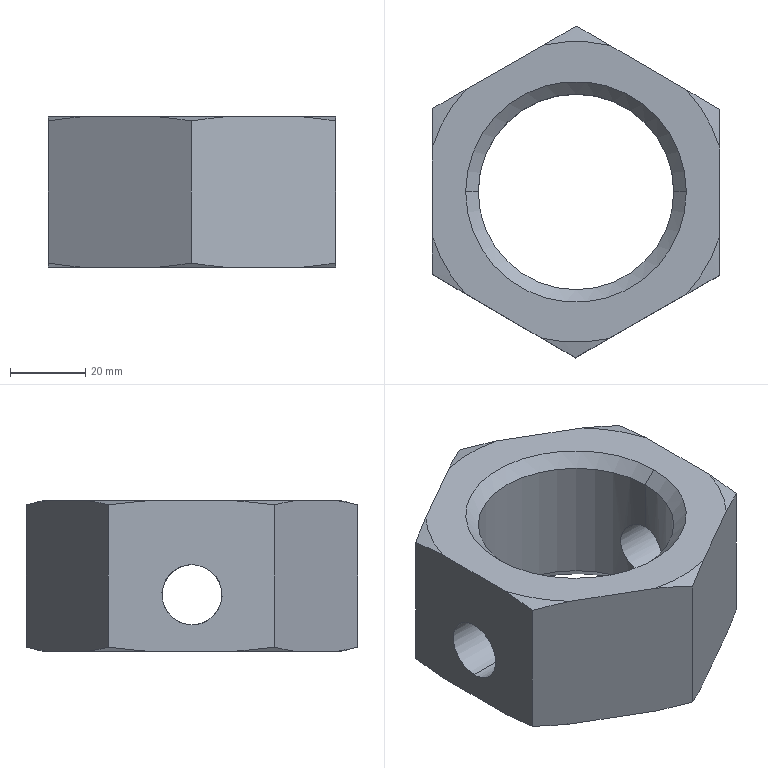Part | NX | features BREP 1 | 1 solid | 30 faces | box 76.6 x 88.249 x 40 mm | volume 110310 mm3 | cone 16 | plane 8 | cylinder 6 | commonest cylinder face diameters 16 x4 52 x2
STEP:
#1=CARTESIAN_POINT('',(-38.214,0.,23.));
#2=VERTEX_POINT('',#1);
#3=CARTESIAN_POINT('',(-38.214,0.,7.));
#4=VERTEX_POINT('',#3);
#5=CARTESIAN_POINT('',(-38.214,0.,23.));
#6=CARTESIAN_POINT('',(-38.277,-16.,23.));
#7=CARTESIAN_POINT('',(-38.277,-16.,7.));
#8=CARTESIAN_POINT('',(-38.214,0.,7.));
#9=(BOUNDED_CURVE()B_SPLINE_CURVE(3,(#5,#6,#7,#8),.UNSPECIFIED.,.F.,.F.)B_SPLINE_CURVE_WITH_KNOTS((4,4),(0.,1.),.PIECEWISE_BEZIER_KNOTS.)CURVE()GEOMETRIC_REPRESENTATION_ITEM()RATIONAL_B_SPLINE_CURVE((1.,0.3333,0.3333,1.))REPRESENTATION_ITEM(''));
#10=EDGE_CURVE('',#2,#4,#9,.T.);
#11=ORIENTED_EDGE('',*,*,#10,.F.);
#12=CARTESIAN_POINT('',(-26.,0.,23.));
#13=VERTEX_POINT('',#12);
#14=CARTESIAN_POINT('',(-60.,0.,23.));
#15=DIRECTION('',(1.,0.,0.));
#16=VECTOR('',#15,1000.);
#17=LINE('',#14,#16);
#18=EDGE_CURVE('',#13,#2,#17,.F.);
#19=ORIENTED_EDGE('',*,*,#18,.F.);
#20=CARTESIAN_POINT('',(-26.,0.,7.));
#21=VERTEX_POINT('',#20);
#22=CARTESIAN_POINT('',(-26.,0.,23.));
#23=CARTESIAN_POINT('',(-26.,-2.127,23.));
#24=CARTESIAN_POINT('',(-25.385,-6.252,21.264));
#25=CARTESIAN_POINT('',(-24.416,-8.873,15.013));
#26=CARTESIAN_POINT('',(-25.384,-6.255,8.732));
#27=CARTESIAN_POINT('',(-26.,-2.128,7.));
#28=CARTESIAN_POINT('',(-26.,0.,7.));
#29=B_SPLINE_CURVE_WITH_KNOTS('',3,(#22,#23,#24,#25,#26,#27,#28),.UNSPECIFIED.,.F.,.F.,(4,1,1,1,4),(0.,0.006289,0.01258,0.01887,0.02516),.UNSPECIFIED.);
#30=EDGE_CURVE('',#13,#21,#29,.T.);
#31=ORIENTED_EDGE('',*,*,#30,.T.);
#32=CARTESIAN_POINT('',(-60.,0.,7.));
#33=DIRECTION('',(1.,0.,0.));
#34=VECTOR('',#33,1000.);
#35=LINE('',#32,#34);
#36=EDGE_CURVE('',#21,#4,#35,.F.);
#37=ORIENTED_EDGE('',*,*,#36,.T.);
#38=EDGE_LOOP('',(#11,#19,#31,#37));
#39=FACE_BOUND('',#38,.T.);
#40=CARTESIAN_POINT('',(-60.,0.,15.));
#41=DIRECTION('',(1.,0.,0.));
#42=DIRECTION('',(0.,0.,1.));
#43=AXIS2_PLACEMENT_3D('',#40,#41,#42);
#44=CYLINDRICAL_SURFACE('',#43,8.);
#45=ADVANCED_FACE('',(#39),#44,.F.);
#46=CARTESIAN_POINT('',(26.,0.,7.));
#47=VERTEX_POINT('',#46);
#48=CARTESIAN_POINT('',(26.,0.,23.));
#49=VERTEX_POINT('',#48);
#50=CARTESIAN_POINT('',(26.,0.,7.));
#51=CARTESIAN_POINT('',(26.,-2.127,7.));
#52=CARTESIAN_POINT('',(25.385,-6.252,8.736));
#53=CARTESIAN_POINT('',(24.416,-8.873,14.987));
#54=CARTESIAN_POINT('',(25.384,-6.255,21.268));
#55=CARTESIAN_POINT('',(26.,-2.128,23.));
#56=CARTESIAN_POINT('',(26.,0.,23.));
#57=B_SPLINE_CURVE_WITH_KNOTS('',3,(#50,#51,#52,#53,#54,#55,#56),.UNSPECIFIED.,.F.,.F.,(4,1,1,1,4),(0.,0.006289,0.01258,0.01887,0.02516),.UNSPECIFIED.);
#58=EDGE_CURVE('',#47,#49,#57,.T.);
#59=ORIENTED_EDGE('',*,*,#58,.T.);
#60=CARTESIAN_POINT('',(38.214,0.,23.));
#61=VERTEX_POINT('',#60);
#62=CARTESIAN_POINT('',(-60.,0.,23.));
#63=DIRECTION('',(1.,0.,0.));
#64=VECTOR('',#63,1000.);
#65=LINE('',#62,#64);
#66=EDGE_CURVE('',#61,#49,#65,.F.);
#67=ORIENTED_EDGE('',*,*,#66,.F.);
#68=CARTESIAN_POINT('',(38.214,0.,7.));
#69=VERTEX_POINT('',#68);
#70=CARTESIAN_POINT('',(38.214,0.,7.));
#71=CARTESIAN_POINT('',(38.151,-16.,7.));
#72=CARTESIAN_POINT('',(38.151,-16.,23.));
#73=CARTESIAN_POINT('',(38.214,0.,23.));
#74=(BOUNDED_CURVE()B_SPLINE_CURVE(3,(#70,#71,#72,#73),.UNSPECIFIED.,.F.,.F.)B_SPLINE_CURVE_WITH_KNOTS((4,4),(0.,1.),.PIECEWISE_BEZIER_KNOTS.)CURVE()GEOMETRIC_REPRESENTATION_ITEM()RATIONAL_B_SPLINE_CURVE((1.,0.3333,0.3333,1.))REPRESENTATION_ITEM(''));
#75=EDGE_CURVE('',#69,#61,#74,.T.);
#76=ORIENTED_EDGE('',*,*,#75,.F.);
#77=CARTESIAN_POINT('',(-60.,0.,7.));
#78=DIRECTION('',(1.,0.,0.));
#79=VECTOR('',#78,1000.);
#80=LINE('',#77,#79);
#81=EDGE_CURVE('',#69,#47,#80,.F.);
#82=ORIENTED_EDGE('',*,*,#81,.T.);
#83=EDGE_LOOP('',(#59,#67,#76,#82));
#84=FACE_BOUND('',#83,.T.);
#85=CARTESIAN_POINT('',(-60.,0.,15.));
#86=DIRECTION('',(1.,0.,0.));
#87=DIRECTION('',(0.,0.,1.));
#88=AXIS2_PLACEMENT_3D('',#85,#86,#87);
#89=CYLINDRICAL_SURFACE('',#88,8.);
#90=ADVANCED_FACE('',(#84),#89,.F.);
#91=CARTESIAN_POINT('',(-26.,0.,36.662));
#92=VERTEX_POINT('',#91);
#93=CARTESIAN_POINT('',(26.,0.,36.662));
#94=VERTEX_POINT('',#93);
#95=CARTESIAN_POINT('',(0.,0.,36.662));
#96=DIRECTION('',(0.,0.,1.));
#97=DIRECTION('',(-1.,0.,0.));
#98=AXIS2_PLACEMENT_3D('',#95,#96,#97);
#99=CIRCLE('',#98,26.);
#100=EDGE_CURVE('',#92,#94,#99,.T.);
#101=ORIENTED_EDGE('',*,*,#100,.F.);
#102=CARTESIAN_POINT('',(-29.338,0.,40.));
#103=VERTEX_POINT('',#102);
#104=CARTESIAN_POINT('',(-26.,0.,36.662));
#105=DIRECTION('',(-0.7071,0.,0.7071));
#106=VECTOR('',#105,1000.);
#107=LINE('',#104,#106);
#108=EDGE_CURVE('',#92,#103,#107,.T.);
#109=ORIENTED_EDGE('',*,*,#108,.T.);
#110=CARTESIAN_POINT('',(29.338,0.,40.));
#111=VERTEX_POINT('',#110);
#112=CARTESIAN_POINT('',(0.,0.,40.));
#113=DIRECTION('',(0.,0.,-1.));
#114=DIRECTION('',(-1.,0.,0.));
#115=AXIS2_PLACEMENT_3D('',#112,#113,#114);
#116=CIRCLE('',#115,29.338);
#117=EDGE_CURVE('',#111,#103,#116,.T.);
#118=ORIENTED_EDGE('',*,*,#117,.F.);
#119=CARTESIAN_POINT('',(26.,0.,36.662));
#120=DIRECTION('',(0.7071,0.,0.7071));
#121=VECTOR('',#120,1000.);
#122=LINE('',#119,#121);
#123=EDGE_CURVE('',#94,#111,#122,.T.);
#124=ORIENTED_EDGE('',*,*,#123,.F.);
#125=EDGE_LOOP('',(#101,#109,#118,#124));
#126=FACE_BOUND('',#125,.T.);
#127=CARTESIAN_POINT('',(0.,0.,36.662));
#128=DIRECTION('',(0.,0.,1.));
#129=DIRECTION('',(-1.,0.,0.));
#130=AXIS2_PLACEMENT_3D('',#127,#128,#129);
#131=CONICAL_SURFACE('',#130,26.,0.7854);
#132=ADVANCED_FACE('',(#126),#131,.F.);
#133=CARTESIAN_POINT('',(26.,0.,3.338));
#134=VERTEX_POINT('',#133);
#135=CARTESIAN_POINT('',(-26.,0.,3.338));
#136=VERTEX_POINT('',#135);
#137=CARTESIAN_POINT('',(0.,0.,3.338));
#138=DIRECTION('',(0.,0.,-1.));
#139=DIRECTION('',(-1.,0.,0.));
#140=AXIS2_PLACEMENT_3D('',#137,#138,#139);
#141=CIRCLE('',#140,26.);
#142=EDGE_CURVE('',#134,#136,#141,.T.);
#143=ORIENTED_EDGE('',*,*,#142,.F.);
#144=CARTESIAN_POINT('',(29.338,0.,0.));
#145=VERTEX_POINT('',#144);
#146=CARTESIAN_POINT('',(29.338,0.,0.));
#147=DIRECTION('',(0.7071,0.,-0.7071));
#148=VECTOR('',#147,1000.);
#149=LINE('',#146,#148);
#150=EDGE_CURVE('',#145,#134,#149,.F.);
#151=ORIENTED_EDGE('',*,*,#150,.F.);
#152=CARTESIAN_POINT('',(-29.338,0.,0.));
#153=VERTEX_POINT('',#152);
#154=CARTESIAN_POINT('',(0.,0.,0.));
#155=DIRECTION('',(0.,0.,1.));
#156=DIRECTION('',(-1.,0.,0.));
#157=AXIS2_PLACEMENT_3D('',#154,#155,#156);
#158=CIRCLE('',#157,29.338);
#159=EDGE_CURVE('',#153,#145,#158,.T.);
#160=ORIENTED_EDGE('',*,*,#159,.F.);
#161=CARTESIAN_POINT('',(-29.338,0.,0.));
#162=DIRECTION('',(-0.7071,0.,-0.7071));
#163=VECTOR('',#162,1000.);
#164=LINE('',#161,#163);
#165=EDGE_CURVE('',#153,#136,#164,.F.);
#166=ORIENTED_EDGE('',*,*,#165,.T.);
#167=EDGE_LOOP('',(#143,#151,#160,#166));
#168=FACE_BOUND('',#167,.T.);
#169=CARTESIAN_POINT('',(0.,0.,0.));
#170=DIRECTION('',(0.,0.,-1.));
#171=DIRECTION('',(1.,0.,0.));
#172=AXIS2_PLACEMENT_3D('',#169,#170,#171);
#173=CONICAL_SURFACE('',#172,29.338,0.7854);
#174=ADVANCED_FACE('',(#168),#173,.F.);
#175=ORIENTED_EDGE('',*,*,#100,.T.);
#176=CARTESIAN_POINT('',(26.,0.,40.));
#177=DIRECTION('',(0.,0.,-1.));
#178=VECTOR('',#177,1000.);
#179=LINE('',#176,#178);
#180=EDGE_CURVE('',#49,#94,#179,.F.);
#181=ORIENTED_EDGE('',*,*,#180,.F.);
#182=ORIENTED_EDGE('',*,*,#58,.F.);
#183=CARTESIAN_POINT('',(26.,0.,40.));
#184=DIRECTION('',(0.,0.,-1.));
#185=VECTOR('',#184,1000.);
#186=LINE('',#183,#185);
#187=EDGE_CURVE('',#134,#47,#186,.F.);
#188=ORIENTED_EDGE('',*,*,#187,.F.);
#189=ORIENTED_EDGE('',*,*,#142,.T.);
#190=CARTESIAN_POINT('',(-26.,0.,40.));
#191=DIRECTION('',(0.,0.,-1.));
#192=VECTOR('',#191,1000.);
#193=LINE('',#190,#192);
#194=EDGE_CURVE('',#136,#21,#193,.F.);
#195=ORIENTED_EDGE('',*,*,#194,.T.);
#196=ORIENTED_EDGE('',*,*,#30,.F.);
#197=CARTESIAN_POINT('',(-26.,0.,40.));
#198=DIRECTION('',(0.,0.,-1.));
#199=VECTOR('',#198,1000.);
#200=LINE('',#197,#199);
#201=EDGE_CURVE('',#13,#92,#200,.F.);
#202=ORIENTED_EDGE('',*,*,#201,.T.);
#203=EDGE_LOOP('',(#175,#181,#182,#188,#189,#195,#196,#202));
#204=FACE_BOUND('',#203,.T.);
#205=CARTESIAN_POINT('',(0.,0.,40.));
#206=DIRECTION('',(0.,0.,-1.));
#207=DIRECTION('',(1.,0.,0.));
#208=AXIS2_PLACEMENT_3D('',#205,#206,#207);
#209=CYLINDRICAL_SURFACE('',#208,26.);
#210=ADVANCED_FACE('',(#204),#209,.F.);
#211=CARTESIAN_POINT('',(38.3,21.912,38.895));
#212=VERTEX_POINT('',#211);
#213=CARTESIAN_POINT('',(29.451,27.068,40.));
#214=VERTEX_POINT('',#213);
#215=CARTESIAN_POINT('',(38.3,21.912,38.895));
#216=CARTESIAN_POINT('',(35.358,23.626,39.351));
#217=CARTESIAN_POINT('',(32.41,25.344,39.729));
#218=CARTESIAN_POINT('',(29.451,27.068,40.));
#219=B_SPLINE_CURVE_WITH_KNOTS('',3,(#215,#216,#217,#218),.UNSPECIFIED.,.F.,.F.,(4,4),(0.,0.0103),.UNSPECIFIED.);
#220=EDGE_CURVE('',#212,#214,#219,.T.);
#221=ORIENTED_EDGE('',*,*,#220,.F.);
#222=CARTESIAN_POINT('',(38.3,21.912,1.105));
#223=VERTEX_POINT('',#222);
#224=CARTESIAN_POINT('',(38.3,21.912,40.));
#225=DIRECTION('',(0.,0.,-1.));
#226=VECTOR('',#225,1000.);
#227=LINE('',#224,#226);
#228=EDGE_CURVE('',#212,#223,#227,.T.);
#229=ORIENTED_EDGE('',*,*,#228,.T.);
#230=CARTESIAN_POINT('',(29.451,27.068,0.));
#231=VERTEX_POINT('',#230);
#232=CARTESIAN_POINT('',(29.451,27.068,0.));
#233=CARTESIAN_POINT('',(32.41,25.344,0.2712));
#234=CARTESIAN_POINT('',(35.358,23.626,0.6492));
#235=CARTESIAN_POINT('',(38.3,21.912,1.105));
#236=B_SPLINE_CURVE_WITH_KNOTS('',3,(#232,#233,#234,#235),.UNSPECIFIED.,.F.,.F.,(4,4),(0.,0.0103),.UNSPECIFIED.);
#237=EDGE_CURVE('',#231,#223,#236,.T.);
#238=ORIENTED_EDGE('',*,*,#237,.F.);
#239=CARTESIAN_POINT('',(9.023,38.969,0.));
#240=VERTEX_POINT('',#239);
#241=CARTESIAN_POINT('',(38.3,21.912,0.));
#242=DIRECTION('',(-0.8641,0.5034,0.));
#243=VECTOR('',#242,1000.);
#244=LINE('',#241,#243);
#245=EDGE_CURVE('',#231,#240,#244,.T.);
#246=ORIENTED_EDGE('',*,*,#245,.T.);
#247=CARTESIAN_POINT('',(0.1736,44.125,1.105));
#248=VERTEX_POINT('',#247);
#249=CARTESIAN_POINT('',(0.1736,44.125,1.105));
#250=CARTESIAN_POINT('',(3.115,42.411,0.6492));
#251=CARTESIAN_POINT('',(6.064,40.693,0.2712));
#252=CARTESIAN_POINT('',(9.023,38.969,0.));
#253=B_SPLINE_CURVE_WITH_KNOTS('',3,(#249,#250,#251,#252),.UNSPECIFIED.,.F.,.F.,(4,4),(0.,0.0103),.UNSPECIFIED.);
#254=EDGE_CURVE('',#248,#240,#253,.T.);
#255=ORIENTED_EDGE('',*,*,#254,.F.);
#256=CARTESIAN_POINT('',(0.1736,44.125,38.895));
#257=VERTEX_POINT('',#256);
#258=CARTESIAN_POINT('',(0.1736,44.125,40.));
#259=DIRECTION('',(0.,0.,-1.));
#260=VECTOR('',#259,1000.);
#261=LINE('',#258,#260);
#262=EDGE_CURVE('',#257,#248,#261,.T.);
#263=ORIENTED_EDGE('',*,*,#262,.F.);
#264=CARTESIAN_POINT('',(9.023,38.969,40.));
#265=VERTEX_POINT('',#264);
#266=CARTESIAN_POINT('',(9.023,38.969,40.));
#267=CARTESIAN_POINT('',(6.064,40.693,39.729));
#268=CARTESIAN_POINT('',(3.115,42.411,39.351));
#269=CARTESIAN_POINT('',(0.1736,44.125,38.895));
#270=B_SPLINE_CURVE_WITH_KNOTS('',3,(#266,#267,#268,#269),.UNSPECIFIED.,.F.,.F.,(4,4),(0.,0.0103),.UNSPECIFIED.);
#271=EDGE_CURVE('',#265,#257,#270,.T.);
#272=ORIENTED_EDGE('',*,*,#271,.F.);
#273=CARTESIAN_POINT('',(38.3,21.912,40.));
#274=DIRECTION('',(-0.8641,0.5034,0.));
#275=VECTOR('',#274,1000.);
#276=LINE('',#273,#275);
#277=EDGE_CURVE('',#214,#265,#276,.T.);
#278=ORIENTED_EDGE('',*,*,#277,.F.);
#279=EDGE_LOOP('',(#221,#229,#238,#246,#255,#263,#272,#278));
#280=FACE_BOUND('',#279,.T.);
#281=CARTESIAN_POINT('',(38.3,21.912,40.));
#282=DIRECTION('',(-0.5034,-0.8641,0.));
#283=DIRECTION('',(-0.8641,0.5034,0.));
#284=AXIS2_PLACEMENT_3D('',#281,#282,#283);
#285=PLANE('',#284);
#286=ADVANCED_FACE('',(#280),#285,.F.);
#287=CARTESIAN_POINT('',(-8.716,39.039,40.));
#288=VERTEX_POINT('',#287);
#289=CARTESIAN_POINT('',(0.1736,44.125,38.895));
#290=CARTESIAN_POINT('',(-2.781,42.434,39.351));
#291=CARTESIAN_POINT('',(-5.744,40.739,39.729));
#292=CARTESIAN_POINT('',(-8.716,39.039,40.));
#293=B_SPLINE_CURVE_WITH_KNOTS('',3,(#289,#290,#291,#292),.UNSPECIFIED.,.F.,.F.,(4,4),(0.,0.0103),.UNSPECIFIED.);
#294=EDGE_CURVE('',#257,#288,#293,.T.);
#295=ORIENTED_EDGE('',*,*,#294,.F.);
#296=ORIENTED_EDGE('',*,*,#262,.T.);
#297=CARTESIAN_POINT('',(-8.716,39.039,0.));
#298=VERTEX_POINT('',#297);
#299=CARTESIAN_POINT('',(-8.716,39.039,0.));
#300=CARTESIAN_POINT('',(-5.744,40.739,0.2712));
#301=CARTESIAN_POINT('',(-2.781,42.434,0.6492));
#302=CARTESIAN_POINT('',(0.1736,44.125,1.105));
#303=B_SPLINE_CURVE_WITH_KNOTS('',3,(#299,#300,#301,#302),.UNSPECIFIED.,.F.,.F.,(4,4),(0.,0.0103),.UNSPECIFIED.);
#304=EDGE_CURVE('',#298,#248,#303,.T.);
#305=ORIENTED_EDGE('',*,*,#304,.F.);
#306=CARTESIAN_POINT('',(-29.237,27.298,0.));
#307=VERTEX_POINT('',#306);
#308=CARTESIAN_POINT('',(0.1736,44.125,0.));
#309=DIRECTION('',(-0.868,-0.4966,0.));
#310=VECTOR('',#309,1000.);
#311=LINE('',#308,#310);
#312=EDGE_CURVE('',#298,#307,#311,.T.);
#313=ORIENTED_EDGE('',*,*,#312,.T.);
#314=CARTESIAN_POINT('',(-38.126,22.213,1.105));
#315=VERTEX_POINT('',#314);
#316=CARTESIAN_POINT('',(-38.126,22.213,1.105));
#317=CARTESIAN_POINT('',(-35.171,23.903,0.6492));
#318=CARTESIAN_POINT('',(-32.209,25.598,0.2712));
#319=CARTESIAN_POINT('',(-29.237,27.298,0.));
#320=B_SPLINE_CURVE_WITH_KNOTS('',3,(#316,#317,#318,#319),.UNSPECIFIED.,.F.,.F.,(4,4),(0.,0.0103),.UNSPECIFIED.);
#321=EDGE_CURVE('',#315,#307,#320,.T.);
#322=ORIENTED_EDGE('',*,*,#321,.F.);
#323=CARTESIAN_POINT('',(-38.126,22.213,38.895));
#324=VERTEX_POINT('',#323);
#325=CARTESIAN_POINT('',(-38.126,22.213,40.));
#326=DIRECTION('',(0.,0.,-1.));
#327=VECTOR('',#326,1000.);
#328=LINE('',#325,#327);
#329=EDGE_CURVE('',#324,#315,#328,.T.);
#330=ORIENTED_EDGE('',*,*,#329,.F.);
#331=CARTESIAN_POINT('',(-29.237,27.298,40.));
#332=VERTEX_POINT('',#331);
#333=CARTESIAN_POINT('',(-29.237,27.298,40.));
#334=CARTESIAN_POINT('',(-32.209,25.598,39.729));
#335=CARTESIAN_POINT('',(-35.171,23.903,39.351));
#336=CARTESIAN_POINT('',(-38.126,22.213,38.895));
#337=B_SPLINE_CURVE_WITH_KNOTS('',3,(#333,#334,#335,#336),.UNSPECIFIED.,.F.,.F.,(4,4),(0.,0.0103),.UNSPECIFIED.);
#338=EDGE_CURVE('',#332,#324,#337,.T.);
#339=ORIENTED_EDGE('',*,*,#338,.F.);
#340=CARTESIAN_POINT('',(0.1736,44.125,40.));
#341=DIRECTION('',(-0.868,-0.4966,0.));
#342=VECTOR('',#341,1000.);
#343=LINE('',#340,#342);
#344=EDGE_CURVE('',#288,#332,#343,.T.);
#345=ORIENTED_EDGE('',*,*,#344,.F.);
#346=EDGE_LOOP('',(#295,#296,#305,#313,#322,#330,#339,#345));
#347=FACE_BOUND('',#346,.T.);
#348=CARTESIAN_POINT('',(0.1736,44.125,40.));
#349=DIRECTION('',(0.4966,-0.868,0.));
#350=DIRECTION('',(-0.868,-0.4966,0.));
#351=AXIS2_PLACEMENT_3D('',#348,#349,#350);
#352=PLANE('',#351);
#353=ADVANCED_FACE('',(#347),#352,.F.);
#354=CARTESIAN_POINT('',(-38.214,0.,7.));
#355=CARTESIAN_POINT('',(-38.151,16.,7.));
#356=CARTESIAN_POINT('',(-38.151,16.,23.));
#357=CARTESIAN_POINT('',(-38.214,0.,23.));
#358=(BOUNDED_CURVE()B_SPLINE_CURVE(3,(#354,#355,#356,#357),.UNSPECIFIED.,.F.,.F.)B_SPLINE_CURVE_WITH_KNOTS((4,4),(0.,1.),.PIECEWISE_BEZIER_KNOTS.)CURVE()GEOMETRIC_REPRESENTATION_ITEM()RATIONAL_B_SPLINE_CURVE((1.,0.3333,0.3333,1.))REPRESENTATION_ITEM(''));
#359=EDGE_CURVE('',#4,#2,#358,.T.);
#360=ORIENTED_EDGE('',*,*,#359,.T.);
#361=ORIENTED_EDGE('',*,*,#10,.T.);
#362=EDGE_LOOP('',(#360,#361));
#363=FACE_BOUND('',#362,.T.);
#364=CARTESIAN_POINT('',(-38.167,11.971,40.));
#365=VERTEX_POINT('',#364);
#366=CARTESIAN_POINT('',(-38.126,22.213,38.895));
#367=CARTESIAN_POINT('',(-38.14,18.808,39.351));
#368=CARTESIAN_POINT('',(-38.153,15.396,39.729));
#369=CARTESIAN_POINT('',(-38.167,11.971,40.));
#370=B_SPLINE_CURVE_WITH_KNOTS('',3,(#366,#367,#368,#369),.UNSPECIFIED.,.F.,.F.,(4,4),(0.,0.0103),.UNSPECIFIED.);
#371=EDGE_CURVE('',#324,#365,#370,.T.);
#372=ORIENTED_EDGE('',*,*,#371,.F.);
#373=ORIENTED_EDGE('',*,*,#329,.T.);
#374=CARTESIAN_POINT('',(-38.167,11.971,0.));
#375=VERTEX_POINT('',#374);
#376=CARTESIAN_POINT('',(-38.167,11.971,0.));
#377=CARTESIAN_POINT('',(-38.153,15.396,0.2712));
#378=CARTESIAN_POINT('',(-38.14,18.808,0.6492));
#379=CARTESIAN_POINT('',(-38.126,22.213,1.105));
#380=B_SPLINE_CURVE_WITH_KNOTS('',3,(#376,#377,#378,#379),.UNSPECIFIED.,.F.,.F.,(4,4),(0.,0.0103),.UNSPECIFIED.);
#381=EDGE_CURVE('',#375,#315,#380,.T.);
#382=ORIENTED_EDGE('',*,*,#381,.F.);
#383=CARTESIAN_POINT('',(-38.26,-11.671,0.));
#384=VERTEX_POINT('',#383);
#385=CARTESIAN_POINT('',(-38.126,22.213,0.));
#386=DIRECTION('',(-0.003934,-1.,0.));
#387=VECTOR('',#386,1000.);
#388=LINE('',#385,#387);
#389=EDGE_CURVE('',#375,#384,#388,.T.);
#390=ORIENTED_EDGE('',*,*,#389,.T.);
#391=CARTESIAN_POINT('',(-38.3,-21.912,1.105));
#392=VERTEX_POINT('',#391);
#393=CARTESIAN_POINT('',(-38.3,-21.912,1.105));
#394=CARTESIAN_POINT('',(-38.286,-18.508,0.6492));
#395=CARTESIAN_POINT('',(-38.273,-15.095,0.2712));
#396=CARTESIAN_POINT('',(-38.26,-11.671,0.));
#397=B_SPLINE_CURVE_WITH_KNOTS('',3,(#393,#394,#395,#396),.UNSPECIFIED.,.F.,.F.,(4,4),(0.,0.0103),.UNSPECIFIED.);
#398=EDGE_CURVE('',#392,#384,#397,.T.);
#399=ORIENTED_EDGE('',*,*,#398,.F.);
#400=CARTESIAN_POINT('',(-38.3,-21.912,38.895));
#401=VERTEX_POINT('',#400);
#402=CARTESIAN_POINT('',(-38.3,-21.912,40.));
#403=DIRECTION('',(0.,0.,-1.));
#404=VECTOR('',#403,1000.);
#405=LINE('',#402,#404);
#406=EDGE_CURVE('',#401,#392,#405,.T.);
#407=ORIENTED_EDGE('',*,*,#406,.F.);
#408=CARTESIAN_POINT('',(-38.26,-11.671,40.));
#409=VERTEX_POINT('',#408);
#410=CARTESIAN_POINT('',(-38.26,-11.671,40.));
#411=CARTESIAN_POINT('',(-38.273,-15.095,39.729));
#412=CARTESIAN_POINT('',(-38.286,-18.508,39.351));
#413=CARTESIAN_POINT('',(-38.3,-21.912,38.895));
#414=B_SPLINE_CURVE_WITH_KNOTS('',3,(#410,#411,#412,#413),.UNSPECIFIED.,.F.,.F.,(4,4),(0.,0.0103),.UNSPECIFIED.);
#415=EDGE_CURVE('',#409,#401,#414,.T.);
#416=ORIENTED_EDGE('',*,*,#415,.F.);
#417=CARTESIAN_POINT('',(-38.126,22.213,40.));
#418=DIRECTION('',(-0.003934,-1.,0.));
#419=VECTOR('',#418,1000.);
#420=LINE('',#417,#419);
#421=EDGE_CURVE('',#365,#409,#420,.T.);
#422=ORIENTED_EDGE('',*,*,#421,.F.);
#423=EDGE_LOOP('',(#372,#373,#382,#390,#399,#407,#416,#422));
#424=FACE_BOUND('',#423,.T.);
#425=CARTESIAN_POINT('',(-38.126,22.213,40.));
#426=DIRECTION('',(1.,-0.003934,0.));
#427=DIRECTION('',(-0.003934,-1.,0.));
#428=AXIS2_PLACEMENT_3D('',#425,#426,#427);
#429=PLANE('',#428);
#430=ADVANCED_FACE('',(#363,#424),#429,.F.);
#431=CARTESIAN_POINT('',(-29.451,-27.068,40.));
#432=VERTEX_POINT('',#431);
#433=CARTESIAN_POINT('',(-38.3,-21.912,38.895));
#434=CARTESIAN_POINT('',(-35.358,-23.626,39.351));
#435=CARTESIAN_POINT('',(-32.41,-25.344,39.729));
#436=CARTESIAN_POINT('',(-29.451,-27.068,40.));
#437=B_SPLINE_CURVE_WITH_KNOTS('',3,(#433,#434,#435,#436),.UNSPECIFIED.,.F.,.F.,(4,4),(0.,0.0103),.UNSPECIFIED.);
#438=EDGE_CURVE('',#401,#432,#437,.T.);
#439=ORIENTED_EDGE('',*,*,#438,.F.);
#440=ORIENTED_EDGE('',*,*,#406,.T.);
#441=CARTESIAN_POINT('',(-29.451,-27.068,0.));
#442=VERTEX_POINT('',#441);
#443=CARTESIAN_POINT('',(-29.451,-27.068,0.));
#444=CARTESIAN_POINT('',(-32.41,-25.344,0.2712));
#445=CARTESIAN_POINT('',(-35.358,-23.626,0.6492));
#446=CARTESIAN_POINT('',(-38.3,-21.912,1.105));
#447=B_SPLINE_CURVE_WITH_KNOTS('',3,(#443,#444,#445,#446),.UNSPECIFIED.,.F.,.F.,(4,4),(0.,0.0103),.UNSPECIFIED.);
#448=EDGE_CURVE('',#442,#392,#447,.T.);
#449=ORIENTED_EDGE('',*,*,#448,.F.);
#450=CARTESIAN_POINT('',(-9.023,-38.969,0.));
#451=VERTEX_POINT('',#450);
#452=CARTESIAN_POINT('',(-38.3,-21.912,0.));
#453=DIRECTION('',(0.8641,-0.5034,0.));
#454=VECTOR('',#453,1000.);
#455=LINE('',#452,#454);
#456=EDGE_CURVE('',#442,#451,#455,.T.);
#457=ORIENTED_EDGE('',*,*,#456,.T.);
#458=CARTESIAN_POINT('',(-0.1736,-44.125,1.105));
#459=VERTEX_POINT('',#458);
#460=CARTESIAN_POINT('',(-0.1736,-44.125,1.105));
#461=CARTESIAN_POINT('',(-3.115,-42.411,0.6492));
#462=CARTESIAN_POINT('',(-6.064,-40.693,0.2712));
#463=CARTESIAN_POINT('',(-9.023,-38.969,0.));
#464=B_SPLINE_CURVE_WITH_KNOTS('',3,(#460,#461,#462,#463),.UNSPECIFIED.,.F.,.F.,(4,4),(0.,0.0103),.UNSPECIFIED.);
#465=EDGE_CURVE('',#459,#451,#464,.T.);
#466=ORIENTED_EDGE('',*,*,#465,.F.);
#467=CARTESIAN_POINT('',(-0.1736,-44.125,38.895));
#468=VERTEX_POINT('',#467);
#469=CARTESIAN_POINT('',(-0.1736,-44.125,40.));
#470=DIRECTION('',(0.,0.,-1.));
#471=VECTOR('',#470,1000.);
#472=LINE('',#469,#471);
#473=EDGE_CURVE('',#468,#459,#472,.T.);
#474=ORIENTED_EDGE('',*,*,#473,.F.);
#475=CARTESIAN_POINT('',(-9.023,-38.969,40.));
#476=VERTEX_POINT('',#475);
#477=CARTESIAN_POINT('',(-9.023,-38.969,40.));
#478=CARTESIAN_POINT('',(-6.064,-40.693,39.729));
#479=CARTESIAN_POINT('',(-3.115,-42.411,39.351));
#480=CARTESIAN_POINT('',(-0.1736,-44.125,38.895));
#481=B_SPLINE_CURVE_WITH_KNOTS('',3,(#477,#478,#479,#480),.UNSPECIFIED.,.F.,.F.,(4,4),(0.,0.0103),.UNSPECIFIED.);
#482=EDGE_CURVE('',#476,#468,#481,.T.);
#483=ORIENTED_EDGE('',*,*,#482,.F.);
#484=CARTESIAN_POINT('',(-38.3,-21.912,40.));
#485=DIRECTION('',(0.8641,-0.5034,0.));
#486=VECTOR('',#485,1000.);
#487=LINE('',#484,#486);
#488=EDGE_CURVE('',#432,#476,#487,.T.);
#489=ORIENTED_EDGE('',*,*,#488,.F.);
#490=EDGE_LOOP('',(#439,#440,#449,#457,#466,#474,#483,#489));
#491=FACE_BOUND('',#490,.T.);
#492=CARTESIAN_POINT('',(-38.3,-21.912,40.));
#493=DIRECTION('',(0.5034,0.8641,0.));
#494=DIRECTION('',(0.8641,-0.5034,0.));
#495=AXIS2_PLACEMENT_3D('',#492,#493,#494);
#496=PLANE('',#495);
#497=ADVANCED_FACE('',(#491),#496,.F.);
#498=CARTESIAN_POINT('',(8.716,-39.039,40.));
#499=VERTEX_POINT('',#498);
#500=CARTESIAN_POINT('',(-0.1736,-44.125,38.895));
#501=CARTESIAN_POINT('',(2.781,-42.434,39.351));
#502=CARTESIAN_POINT('',(5.744,-40.739,39.729));
#503=CARTESIAN_POINT('',(8.716,-39.039,40.));
#504=B_SPLINE_CURVE_WITH_KNOTS('',3,(#500,#501,#502,#503),.UNSPECIFIED.,.F.,.F.,(4,4),(0.,0.0103),.UNSPECIFIED.);
#505=EDGE_CURVE('',#468,#499,#504,.T.);
#506=ORIENTED_EDGE('',*,*,#505,.F.);
#507=ORIENTED_EDGE('',*,*,#473,.T.);
#508=CARTESIAN_POINT('',(8.716,-39.039,0.));
#509=VERTEX_POINT('',#508);
#510=CARTESIAN_POINT('',(8.716,-39.039,0.));
#511=CARTESIAN_POINT('',(5.744,-40.739,0.2712));
#512=CARTESIAN_POINT('',(2.781,-42.434,0.6492));
#513=CARTESIAN_POINT('',(-0.1736,-44.125,1.105));
#514=B_SPLINE_CURVE_WITH_KNOTS('',3,(#510,#511,#512,#513),.UNSPECIFIED.,.F.,.F.,(4,4),(0.,0.0103),.UNSPECIFIED.);
#515=EDGE_CURVE('',#509,#459,#514,.T.);
#516=ORIENTED_EDGE('',*,*,#515,.F.);
#517=CARTESIAN_POINT('',(29.237,-27.298,0.));
#518=VERTEX_POINT('',#517);
#519=CARTESIAN_POINT('',(-0.1736,-44.125,0.));
#520=DIRECTION('',(0.868,0.4966,0.));
#521=VECTOR('',#520,1000.);
#522=LINE('',#519,#521);
#523=EDGE_CURVE('',#509,#518,#522,.T.);
#524=ORIENTED_EDGE('',*,*,#523,.T.);
#525=CARTESIAN_POINT('',(38.126,-22.213,1.105));
#526=VERTEX_POINT('',#525);
#527=CARTESIAN_POINT('',(38.126,-22.213,1.105));
#528=CARTESIAN_POINT('',(35.171,-23.903,0.6492));
#529=CARTESIAN_POINT('',(32.209,-25.598,0.2712));
#530=CARTESIAN_POINT('',(29.237,-27.298,0.));
#531=B_SPLINE_CURVE_WITH_KNOTS('',3,(#527,#528,#529,#530),.UNSPECIFIED.,.F.,.F.,(4,4),(0.,0.0103),.UNSPECIFIED.);
#532=EDGE_CURVE('',#526,#518,#531,.T.);
#533=ORIENTED_EDGE('',*,*,#532,.F.);
#534=CARTESIAN_POINT('',(38.126,-22.213,38.895));
#535=VERTEX_POINT('',#534);
#536=CARTESIAN_POINT('',(38.126,-22.213,40.));
#537=DIRECTION('',(0.,0.,-1.));
#538=VECTOR('',#537,1000.);
#539=LINE('',#536,#538);
#540=EDGE_CURVE('',#535,#526,#539,.T.);
#541=ORIENTED_EDGE('',*,*,#540,.F.);
#542=CARTESIAN_POINT('',(29.237,-27.298,40.));
#543=VERTEX_POINT('',#542);
#544=CARTESIAN_POINT('',(29.237,-27.298,40.));
#545=CARTESIAN_POINT('',(32.209,-25.598,39.729));
#546=CARTESIAN_POINT('',(35.171,-23.903,39.351));
#547=CARTESIAN_POINT('',(38.126,-22.213,38.895));
#548=B_SPLINE_CURVE_WITH_KNOTS('',3,(#544,#545,#546,#547),.UNSPECIFIED.,.F.,.F.,(4,4),(0.,0.0103),.UNSPECIFIED.);
#549=EDGE_CURVE('',#543,#535,#548,.T.);
#550=ORIENTED_EDGE('',*,*,#549,.F.);
#551=CARTESIAN_POINT('',(-0.1736,-44.125,40.));
#552=DIRECTION('',(0.868,0.4966,0.));
#553=VECTOR('',#552,1000.);
#554=LINE('',#551,#553);
#555=EDGE_CURVE('',#499,#543,#554,.T.);
#556=ORIENTED_EDGE('',*,*,#555,.F.);
#557=EDGE_LOOP('',(#506,#507,#516,#524,#533,#541,#550,#556));
#558=FACE_BOUND('',#557,.T.);
#559=CARTESIAN_POINT('',(-0.1736,-44.125,40.));
#560=DIRECTION('',(-0.4966,0.868,0.));
#561=DIRECTION('',(0.868,0.4966,0.));
#562=AXIS2_PLACEMENT_3D('',#559,#560,#561);
#563=PLANE('',#562);
#564=ADVANCED_FACE('',(#558),#563,.F.);
#565=ORIENTED_EDGE('',*,*,#75,.T.);
#566=CARTESIAN_POINT('',(38.214,0.,23.));
#567=CARTESIAN_POINT('',(38.277,16.,23.));
#568=CARTESIAN_POINT('',(38.277,16.,7.));
#569=CARTESIAN_POINT('',(38.214,0.,7.));
#570=(BOUNDED_CURVE()B_SPLINE_CURVE(3,(#566,#567,#568,#569),.UNSPECIFIED.,.F.,.F.)B_SPLINE_CURVE_WITH_KNOTS((4,4),(0.,1.),.PIECEWISE_BEZIER_KNOTS.)CURVE()GEOMETRIC_REPRESENTATION_ITEM()RATIONAL_B_SPLINE_CURVE((1.,0.3333,0.3333,1.))REPRESENTATION_ITEM(''));
#571=EDGE_CURVE('',#61,#69,#570,.T.);
#572=ORIENTED_EDGE('',*,*,#571,.T.);
#573=EDGE_LOOP('',(#565,#572));
#574=FACE_BOUND('',#573,.T.);
#575=CARTESIAN_POINT('',(38.167,-11.971,40.));
#576=VERTEX_POINT('',#575);
#577=CARTESIAN_POINT('',(38.126,-22.213,38.895));
#578=CARTESIAN_POINT('',(38.14,-18.808,39.351));
#579=CARTESIAN_POINT('',(38.153,-15.396,39.729));
#580=CARTESIAN_POINT('',(38.167,-11.971,40.));
#581=B_SPLINE_CURVE_WITH_KNOTS('',3,(#577,#578,#579,#580),.UNSPECIFIED.,.F.,.F.,(4,4),(0.,0.0103),.UNSPECIFIED.);
#582=EDGE_CURVE('',#535,#576,#581,.T.);
#583=ORIENTED_EDGE('',*,*,#582,.F.);
#584=ORIENTED_EDGE('',*,*,#540,.T.);
#585=CARTESIAN_POINT('',(38.167,-11.971,0.));
#586=VERTEX_POINT('',#585);
#587=CARTESIAN_POINT('',(38.167,-11.971,0.));
#588=CARTESIAN_POINT('',(38.153,-15.396,0.2712));
#589=CARTESIAN_POINT('',(38.14,-18.808,0.6492));
#590=CARTESIAN_POINT('',(38.126,-22.213,1.105));
#591=B_SPLINE_CURVE_WITH_KNOTS('',3,(#587,#588,#589,#590),.UNSPECIFIED.,.F.,.F.,(4,4),(0.,0.0103),.UNSPECIFIED.);
#592=EDGE_CURVE('',#586,#526,#591,.T.);
#593=ORIENTED_EDGE('',*,*,#592,.F.);
#594=CARTESIAN_POINT('',(38.26,11.671,0.));
#595=VERTEX_POINT('',#594);
#596=CARTESIAN_POINT('',(38.126,-22.213,0.));
#597=DIRECTION('',(0.003934,1.,0.));
#598=VECTOR('',#597,1000.);
#599=LINE('',#596,#598);
#600=EDGE_CURVE('',#586,#595,#599,.T.);
#601=ORIENTED_EDGE('',*,*,#600,.T.);
#602=CARTESIAN_POINT('',(38.3,21.912,1.105));
#603=CARTESIAN_POINT('',(38.286,18.508,0.6492));
#604=CARTESIAN_POINT('',(38.273,15.095,0.2712));
#605=CARTESIAN_POINT('',(38.26,11.671,0.));
#606=B_SPLINE_CURVE_WITH_KNOTS('',3,(#602,#603,#604,#605),.UNSPECIFIED.,.F.,.F.,(4,4),(0.,0.0103),.UNSPECIFIED.);
#607=EDGE_CURVE('',#223,#595,#606,.T.);
#608=ORIENTED_EDGE('',*,*,#607,.F.);
#609=ORIENTED_EDGE('',*,*,#228,.F.);
#610=CARTESIAN_POINT('',(38.26,11.671,40.));
#611=VERTEX_POINT('',#610);
#612=CARTESIAN_POINT('',(38.26,11.671,40.));
#613=CARTESIAN_POINT('',(38.273,15.095,39.729));
#614=CARTESIAN_POINT('',(38.286,18.508,39.351));
#615=CARTESIAN_POINT('',(38.3,21.912,38.895));
#616=B_SPLINE_CURVE_WITH_KNOTS('',3,(#612,#613,#614,#615),.UNSPECIFIED.,.F.,.F.,(4,4),(0.,0.0103),.UNSPECIFIED.);
#617=EDGE_CURVE('',#611,#212,#616,.T.);
#618=ORIENTED_EDGE('',*,*,#617,.F.);
#619=CARTESIAN_POINT('',(38.126,-22.213,40.));
#620=DIRECTION('',(0.003934,1.,0.));
#621=VECTOR('',#620,1000.);
#622=LINE('',#619,#621);
#623=EDGE_CURVE('',#576,#611,#622,.T.);
#624=ORIENTED_EDGE('',*,*,#623,.F.);
#625=EDGE_LOOP('',(#583,#584,#593,#601,#608,#609,#618,#624));
#626=FACE_BOUND('',#625,.T.);
#627=CARTESIAN_POINT('',(38.126,-22.213,40.));
#628=DIRECTION('',(-1.,0.003934,0.));
#629=DIRECTION('',(0.003934,1.,0.));
#630=AXIS2_PLACEMENT_3D('',#627,#628,#629);
#631=PLANE('',#630);
#632=ADVANCED_FACE('',(#574,#626),#631,.F.);
#633=ORIENTED_EDGE('',*,*,#117,.T.);
#634=CARTESIAN_POINT('',(0.,0.,40.));
#635=DIRECTION('',(0.,0.,-1.));
#636=DIRECTION('',(-1.,0.,0.));
#637=AXIS2_PLACEMENT_3D('',#634,#635,#636);
#638=CIRCLE('',#637,29.338);
#639=EDGE_CURVE('',#103,#111,#638,.T.);
#640=ORIENTED_EDGE('',*,*,#639,.T.);
#641=EDGE_LOOP('',(#633,#640));
#642=FACE_BOUND('',#641,.T.);
#643=CARTESIAN_POINT('',(0.,0.,40.));
#644=DIRECTION('',(0.,0.,-1.));
#645=DIRECTION('',(-1.,0.,0.));
#646=AXIS2_PLACEMENT_3D('',#643,#644,#645);
#647=CIRCLE('',#646,40.);
#648=EDGE_CURVE('',#365,#332,#647,.T.);
#649=ORIENTED_EDGE('',*,*,#648,.F.);
#650=ORIENTED_EDGE('',*,*,#421,.T.);
#651=CARTESIAN_POINT('',(0.,0.,40.));
#652=DIRECTION('',(0.,0.,-1.));
#653=DIRECTION('',(-1.,0.,0.));
#654=AXIS2_PLACEMENT_3D('',#651,#652,#653);
#655=CIRCLE('',#654,40.);
#656=EDGE_CURVE('',#432,#409,#655,.T.);
#657=ORIENTED_EDGE('',*,*,#656,.F.);
#658=ORIENTED_EDGE('',*,*,#488,.T.);
#659=CARTESIAN_POINT('',(0.,0.,40.));
#660=DIRECTION('',(0.,0.,-1.));
#661=DIRECTION('',(-1.,0.,0.));
#662=AXIS2_PLACEMENT_3D('',#659,#660,#661);
#663=CIRCLE('',#662,40.);
#664=EDGE_CURVE('',#499,#476,#663,.T.);
#665=ORIENTED_EDGE('',*,*,#664,.F.);
#666=ORIENTED_EDGE('',*,*,#555,.T.);
#667=CARTESIAN_POINT('',(0.,0.,40.));
#668=DIRECTION('',(0.,0.,-1.));
#669=DIRECTION('',(-1.,0.,0.));
#670=AXIS2_PLACEMENT_3D('',#667,#668,#669);
#671=CIRCLE('',#670,40.);
#672=EDGE_CURVE('',#576,#543,#671,.T.);
#673=ORIENTED_EDGE('',*,*,#672,.F.);
#674=ORIENTED_EDGE('',*,*,#623,.T.);
#675=CARTESIAN_POINT('',(0.,0.,40.));
#676=DIRECTION('',(0.,0.,1.));
#677=DIRECTION('',(1.,0.,0.));
#678=AXIS2_PLACEMENT_3D('',#675,#676,#677);
#679=CIRCLE('',#678,40.);
#680=EDGE_CURVE('',#611,#214,#679,.T.);
#681=ORIENTED_EDGE('',*,*,#680,.T.);
#682=ORIENTED_EDGE('',*,*,#277,.T.);
#683=CARTESIAN_POINT('',(0.,0.,40.));
#684=DIRECTION('',(0.,0.,-1.));
#685=DIRECTION('',(-1.,0.,0.));
#686=AXIS2_PLACEMENT_3D('',#683,#684,#685);
#687=CIRCLE('',#686,40.);
#688=EDGE_CURVE('',#288,#265,#687,.T.);
#689=ORIENTED_EDGE('',*,*,#688,.F.);
#690=ORIENTED_EDGE('',*,*,#344,.T.);
#691=EDGE_LOOP('',(#649,#650,#657,#658,#665,#666,#673,#674,#681,#682,#689,#690));
#692=FACE_BOUND('',#691,.T.);
#693=CARTESIAN_POINT('',(76.426,-0.3006,40.));
#694=DIRECTION('',(0.,0.,-1.));
#695=DIRECTION('',(1.,0.,0.));
#696=AXIS2_PLACEMENT_3D('',#693,#694,#695);
#697=PLANE('',#696);
#698=ADVANCED_FACE('',(#642,#692),#697,.F.);
#699=ORIENTED_EDGE('',*,*,#159,.T.);
#700=CARTESIAN_POINT('',(0.,0.,0.));
#701=DIRECTION('',(0.,0.,1.));
#702=DIRECTION('',(-1.,0.,0.));
#703=AXIS2_PLACEMENT_3D('',#700,#701,#702);
#704=CIRCLE('',#703,29.338);
#705=EDGE_CURVE('',#145,#153,#704,.T.);
#706=ORIENTED_EDGE('',*,*,#705,.T.);
#707=EDGE_LOOP('',(#699,#706));
#708=FACE_BOUND('',#707,.T.);
#709=ORIENTED_EDGE('',*,*,#389,.F.);
#710=CARTESIAN_POINT('',(0.,0.,0.));
#711=DIRECTION('',(0.,0.,-1.));
#712=DIRECTION('',(-1.,0.,0.));
#713=AXIS2_PLACEMENT_3D('',#710,#711,#712);
#714=CIRCLE('',#713,40.);
#715=EDGE_CURVE('',#375,#307,#714,.T.);
#716=ORIENTED_EDGE('',*,*,#715,.T.);
#717=ORIENTED_EDGE('',*,*,#312,.F.);
#718=CARTESIAN_POINT('',(0.,0.,0.));
#719=DIRECTION('',(0.,0.,-1.));
#720=DIRECTION('',(-1.,0.,0.));
#721=AXIS2_PLACEMENT_3D('',#718,#719,#720);
#722=CIRCLE('',#721,40.);
#723=EDGE_CURVE('',#298,#240,#722,.T.);
#724=ORIENTED_EDGE('',*,*,#723,.T.);
#725=ORIENTED_EDGE('',*,*,#245,.F.);
#726=CARTESIAN_POINT('',(0.,0.,0.));
#727=DIRECTION('',(0.,0.,-1.));
#728=DIRECTION('',(-1.,0.,0.));
#729=AXIS2_PLACEMENT_3D('',#726,#727,#728);
#730=CIRCLE('',#729,40.);
#731=EDGE_CURVE('',#231,#595,#730,.T.);
#732=ORIENTED_EDGE('',*,*,#731,.T.);
#733=ORIENTED_EDGE('',*,*,#600,.F.);
#734=CARTESIAN_POINT('',(0.,0.,0.));
#735=DIRECTION('',(0.,0.,-1.));
#736=DIRECTION('',(-1.,0.,0.));
#737=AXIS2_PLACEMENT_3D('',#734,#735,#736);
#738=CIRCLE('',#737,40.);
#739=EDGE_CURVE('',#586,#518,#738,.T.);
#740=ORIENTED_EDGE('',*,*,#739,.T.);
#741=ORIENTED_EDGE('',*,*,#523,.F.);
#742=CARTESIAN_POINT('',(0.,0.,0.));
#743=DIRECTION('',(0.,0.,-1.));
#744=DIRECTION('',(-1.,0.,0.));
#745=AXIS2_PLACEMENT_3D('',#742,#743,#744);
#746=CIRCLE('',#745,40.);
#747=EDGE_CURVE('',#509,#451,#746,.T.);
#748=ORIENTED_EDGE('',*,*,#747,.T.);
#749=ORIENTED_EDGE('',*,*,#456,.F.);
#750=CARTESIAN_POINT('',(0.,0.,0.));
#751=DIRECTION('',(0.,0.,-1.));
#752=DIRECTION('',(-1.,0.,0.));
#753=AXIS2_PLACEMENT_3D('',#750,#751,#752);
#754=CIRCLE('',#753,40.);
#755=EDGE_CURVE('',#442,#384,#754,.T.);
#756=ORIENTED_EDGE('',*,*,#755,.T.);
#757=EDGE_LOOP('',(#709,#716,#717,#724,#725,#732,#733,#740,#741,#748,#749,#756));
#758=FACE_BOUND('',#757,.T.);
#759=CARTESIAN_POINT('',(76.426,-0.3006,0.));
#760=DIRECTION('',(0.,0.,-1.));
#761=DIRECTION('',(1.,0.,0.));
#762=AXIS2_PLACEMENT_3D('',#759,#760,#761);
#763=PLANE('',#762);
#764=ADVANCED_FACE('',(#708,#758),#763,.T.);
#765=ORIENTED_EDGE('',*,*,#180,.T.);
#766=CARTESIAN_POINT('',(0.,0.,36.662));
#767=DIRECTION('',(0.,0.,1.));
#768=DIRECTION('',(-1.,0.,0.));
#769=AXIS2_PLACEMENT_3D('',#766,#767,#768);
#770=CIRCLE('',#769,26.);
#771=EDGE_CURVE('',#94,#92,#770,.T.);
#772=ORIENTED_EDGE('',*,*,#771,.T.);
#773=ORIENTED_EDGE('',*,*,#201,.F.);
#774=CARTESIAN_POINT('',(-26.,0.,7.));
#775=CARTESIAN_POINT('',(-26.,2.127,7.));
#776=CARTESIAN_POINT('',(-25.385,6.252,8.736));
#777=CARTESIAN_POINT('',(-24.416,8.873,14.987));
#778=CARTESIAN_POINT('',(-25.384,6.255,21.268));
#779=CARTESIAN_POINT('',(-26.,2.128,23.));
#780=CARTESIAN_POINT('',(-26.,0.,23.));
#781=B_SPLINE_CURVE_WITH_KNOTS('',3,(#774,#775,#776,#777,#778,#779,#780),.UNSPECIFIED.,.F.,.F.,(4,1,1,1,4),(0.,0.006289,0.01258,0.01887,0.02516),.UNSPECIFIED.);
#782=EDGE_CURVE('',#21,#13,#781,.T.);
#783=ORIENTED_EDGE('',*,*,#782,.F.);
#784=ORIENTED_EDGE('',*,*,#194,.F.);
#785=CARTESIAN_POINT('',(0.,0.,3.338));
#786=DIRECTION('',(0.,0.,-1.));
#787=DIRECTION('',(-1.,0.,0.));
#788=AXIS2_PLACEMENT_3D('',#785,#786,#787);
#789=CIRCLE('',#788,26.);
#790=EDGE_CURVE('',#136,#134,#789,.T.);
#791=ORIENTED_EDGE('',*,*,#790,.T.);
#792=ORIENTED_EDGE('',*,*,#187,.T.);
#793=CARTESIAN_POINT('',(26.,0.,23.));
#794=CARTESIAN_POINT('',(26.,2.127,23.));
#795=CARTESIAN_POINT('',(25.385,6.252,21.264));
#796=CARTESIAN_POINT('',(24.416,8.873,15.013));
#797=CARTESIAN_POINT('',(25.384,6.255,8.732));
#798=CARTESIAN_POINT('',(26.,2.128,7.));
#799=CARTESIAN_POINT('',(26.,0.,7.));
#800=B_SPLINE_CURVE_WITH_KNOTS('',3,(#793,#794,#795,#796,#797,#798,#799),.UNSPECIFIED.,.F.,.F.,(4,1,1,1,4),(0.,0.006289,0.01258,0.01887,0.02516),.UNSPECIFIED.);
#801=EDGE_CURVE('',#49,#47,#800,.T.);
#802=ORIENTED_EDGE('',*,*,#801,.F.);
#803=EDGE_LOOP('',(#765,#772,#773,#783,#784,#791,#792,#802));
#804=FACE_BOUND('',#803,.T.);
#805=CARTESIAN_POINT('',(0.,0.,40.));
#806=DIRECTION('',(0.,0.,-1.));
#807=DIRECTION('',(1.,0.,0.));
#808=AXIS2_PLACEMENT_3D('',#805,#806,#807);
#809=CYLINDRICAL_SURFACE('',#808,26.);
#810=ADVANCED_FACE('',(#804),#809,.F.);
#811=ORIENTED_EDGE('',*,*,#532,.T.);
#812=ORIENTED_EDGE('',*,*,#739,.F.);
#813=ORIENTED_EDGE('',*,*,#592,.T.);
#814=EDGE_LOOP('',(#811,#812,#813));
#815=FACE_BOUND('',#814,.T.);
#816=CARTESIAN_POINT('',(0.,0.,0.));
#817=DIRECTION('',(0.,0.,1.));
#818=DIRECTION('',(1.,0.,0.));
#819=AXIS2_PLACEMENT_3D('',#816,#817,#818);
#820=CONICAL_SURFACE('',#819,40.,1.309);
#821=ADVANCED_FACE('',(#815),#820,.T.);
#822=ORIENTED_EDGE('',*,*,#237,.T.);
#823=ORIENTED_EDGE('',*,*,#607,.T.);
#824=ORIENTED_EDGE('',*,*,#731,.F.);
#825=EDGE_LOOP('',(#822,#823,#824));
#826=FACE_BOUND('',#825,.T.);
#827=CARTESIAN_POINT('',(0.,0.,0.));
#828=DIRECTION('',(0.,0.,1.));
#829=DIRECTION('',(1.,0.,0.));
#830=AXIS2_PLACEMENT_3D('',#827,#828,#829);
#831=CONICAL_SURFACE('',#830,40.,1.309);
#832=ADVANCED_FACE('',(#826),#831,.T.);
#833=ORIENTED_EDGE('',*,*,#465,.T.);
#834=ORIENTED_EDGE('',*,*,#747,.F.);
#835=ORIENTED_EDGE('',*,*,#515,.T.);
#836=EDGE_LOOP('',(#833,#834,#835));
#837=FACE_BOUND('',#836,.T.);
#838=CARTESIAN_POINT('',(0.,0.,0.));
#839=DIRECTION('',(0.,0.,1.));
#840=DIRECTION('',(1.,0.,0.));
#841=AXIS2_PLACEMENT_3D('',#838,#839,#840);
#842=CONICAL_SURFACE('',#841,40.,1.309);
#843=ADVANCED_FACE('',(#837),#842,.T.);
#844=ORIENTED_EDGE('',*,*,#398,.T.);
#845=ORIENTED_EDGE('',*,*,#755,.F.);
#846=ORIENTED_EDGE('',*,*,#448,.T.);
#847=EDGE_LOOP('',(#844,#845,#846));
#848=FACE_BOUND('',#847,.T.);
#849=CARTESIAN_POINT('',(0.,0.,0.));
#850=DIRECTION('',(0.,0.,1.));
#851=DIRECTION('',(1.,0.,0.));
#852=AXIS2_PLACEMENT_3D('',#849,#850,#851);
#853=CONICAL_SURFACE('',#852,40.,1.309);
#854=ADVANCED_FACE('',(#848),#853,.T.);
#855=ORIENTED_EDGE('',*,*,#321,.T.);
#856=ORIENTED_EDGE('',*,*,#715,.F.);
#857=ORIENTED_EDGE('',*,*,#381,.T.);
#858=EDGE_LOOP('',(#855,#856,#857));
#859=FACE_BOUND('',#858,.T.);
#860=CARTESIAN_POINT('',(0.,0.,0.));
#861=DIRECTION('',(0.,0.,1.));
#862=DIRECTION('',(1.,0.,0.));
#863=AXIS2_PLACEMENT_3D('',#860,#861,#862);
#864=CONICAL_SURFACE('',#863,40.,1.309);
#865=ADVANCED_FACE('',(#859),#864,.T.);
#866=ORIENTED_EDGE('',*,*,#254,.T.);
#867=ORIENTED_EDGE('',*,*,#723,.F.);
#868=ORIENTED_EDGE('',*,*,#304,.T.);
#869=EDGE_LOOP('',(#866,#867,#868));
#870=FACE_BOUND('',#869,.T.);
#871=CARTESIAN_POINT('',(0.,0.,0.));
#872=DIRECTION('',(0.,0.,1.));
#873=DIRECTION('',(1.,0.,0.));
#874=AXIS2_PLACEMENT_3D('',#871,#872,#873);
#875=CONICAL_SURFACE('',#874,40.,1.309);
#876=ADVANCED_FACE('',(#870),#875,.T.);
#877=ORIENTED_EDGE('',*,*,#415,.T.);
#878=ORIENTED_EDGE('',*,*,#438,.T.);
#879=ORIENTED_EDGE('',*,*,#656,.T.);
#880=EDGE_LOOP('',(#877,#878,#879));
#881=FACE_BOUND('',#880,.T.);
#882=CARTESIAN_POINT('',(0.,0.,40.));
#883=DIRECTION('',(0.,0.,-1.));
#884=DIRECTION('',(-1.,0.,0.));
#885=AXIS2_PLACEMENT_3D('',#882,#883,#884);
#886=CONICAL_SURFACE('',#885,40.,1.309);
#887=ADVANCED_FACE('',(#881),#886,.T.);
#888=ORIENTED_EDGE('',*,*,#482,.T.);
#889=ORIENTED_EDGE('',*,*,#505,.T.);
#890=ORIENTED_EDGE('',*,*,#664,.T.);
#891=EDGE_LOOP('',(#888,#889,#890));
#892=FACE_BOUND('',#891,.T.);
#893=CARTESIAN_POINT('',(0.,0.,40.));
#894=DIRECTION('',(0.,0.,-1.));
#895=DIRECTION('',(-1.,0.,0.));
#896=AXIS2_PLACEMENT_3D('',#893,#894,#895);
#897=CONICAL_SURFACE('',#896,40.,1.309);
#898=ADVANCED_FACE('',(#892),#897,.T.);
#899=ORIENTED_EDGE('',*,*,#549,.T.);
#900=ORIENTED_EDGE('',*,*,#582,.T.);
#901=ORIENTED_EDGE('',*,*,#672,.T.);
#902=EDGE_LOOP('',(#899,#900,#901));
#903=FACE_BOUND('',#902,.T.);
#904=CARTESIAN_POINT('',(0.,0.,40.));
#905=DIRECTION('',(0.,0.,-1.));
#906=DIRECTION('',(-1.,0.,0.));
#907=AXIS2_PLACEMENT_3D('',#904,#905,#906);
#908=CONICAL_SURFACE('',#907,40.,1.309);
#909=ADVANCED_FACE('',(#903),#908,.T.);
#910=ORIENTED_EDGE('',*,*,#220,.T.);
#911=ORIENTED_EDGE('',*,*,#680,.F.);
#912=ORIENTED_EDGE('',*,*,#617,.T.);
#913=EDGE_LOOP('',(#910,#911,#912));
#914=FACE_BOUND('',#913,.T.);
#915=CARTESIAN_POINT('',(0.,0.,40.));
#916=DIRECTION('',(0.,0.,-1.));
#917=DIRECTION('',(-1.,0.,0.));
#918=AXIS2_PLACEMENT_3D('',#915,#916,#917);
#919=CONICAL_SURFACE('',#918,40.,1.309);
#920=ADVANCED_FACE('',(#914),#919,.T.);
#921=ORIENTED_EDGE('',*,*,#271,.T.);
#922=ORIENTED_EDGE('',*,*,#294,.T.);
#923=ORIENTED_EDGE('',*,*,#688,.T.);
#924=EDGE_LOOP('',(#921,#922,#923));
#925=FACE_BOUND('',#924,.T.);
#926=CARTESIAN_POINT('',(0.,0.,40.));
#927=DIRECTION('',(0.,0.,-1.));
#928=DIRECTION('',(-1.,0.,0.));
#929=AXIS2_PLACEMENT_3D('',#926,#927,#928);
#930=CONICAL_SURFACE('',#929,40.,1.309);
#931=ADVANCED_FACE('',(#925),#930,.T.);
#932=ORIENTED_EDGE('',*,*,#338,.T.);
#933=ORIENTED_EDGE('',*,*,#371,.T.);
#934=ORIENTED_EDGE('',*,*,#648,.T.);
#935=EDGE_LOOP('',(#932,#933,#934));
#936=FACE_BOUND('',#935,.T.);
#937=CARTESIAN_POINT('',(0.,0.,40.));
#938=DIRECTION('',(0.,0.,-1.));
#939=DIRECTION('',(-1.,0.,0.));
#940=AXIS2_PLACEMENT_3D('',#937,#938,#939);
#941=CONICAL_SURFACE('',#940,40.,1.309);
#942=ADVANCED_FACE('',(#936),#941,.T.);
#943=ORIENTED_EDGE('',*,*,#150,.T.);
#944=ORIENTED_EDGE('',*,*,#790,.F.);
#945=ORIENTED_EDGE('',*,*,#165,.F.);
#946=ORIENTED_EDGE('',*,*,#705,.F.);
#947=EDGE_LOOP('',(#943,#944,#945,#946));
#948=FACE_BOUND('',#947,.T.);
#949=CARTESIAN_POINT('',(0.,0.,0.));
#950=DIRECTION('',(0.,0.,-1.));
#951=DIRECTION('',(1.,0.,0.));
#952=AXIS2_PLACEMENT_3D('',#949,#950,#951);
#953=CONICAL_SURFACE('',#952,29.338,0.7854);
#954=ADVANCED_FACE('',(#948),#953,.F.);
#955=ORIENTED_EDGE('',*,*,#108,.F.);
#956=ORIENTED_EDGE('',*,*,#771,.F.);
#957=ORIENTED_EDGE('',*,*,#123,.T.);
#958=ORIENTED_EDGE('',*,*,#639,.F.);
#959=EDGE_LOOP('',(#955,#956,#957,#958));
#960=FACE_BOUND('',#959,.T.);
#961=CARTESIAN_POINT('',(0.,0.,36.662));
#962=DIRECTION('',(0.,0.,1.));
#963=DIRECTION('',(-1.,0.,0.));
#964=AXIS2_PLACEMENT_3D('',#961,#962,#963);
#965=CONICAL_SURFACE('',#964,26.,0.7854);
#966=ADVANCED_FACE('',(#960),#965,.F.);
#967=ORIENTED_EDGE('',*,*,#66,.T.);
#968=ORIENTED_EDGE('',*,*,#801,.T.);
#969=ORIENTED_EDGE('',*,*,#81,.F.);
#970=ORIENTED_EDGE('',*,*,#571,.F.);
#971=EDGE_LOOP('',(#967,#968,#969,#970));
#972=FACE_BOUND('',#971,.T.);
#973=CARTESIAN_POINT('',(-60.,0.,15.));
#974=DIRECTION('',(1.,0.,0.));
#975=DIRECTION('',(0.,0.,1.));
#976=AXIS2_PLACEMENT_3D('',#973,#974,#975);
#977=CYLINDRICAL_SURFACE('',#976,8.);
#978=ADVANCED_FACE('',(#972),#977,.F.);
#979=ORIENTED_EDGE('',*,*,#18,.T.);
#980=ORIENTED_EDGE('',*,*,#359,.F.);
#981=ORIENTED_EDGE('',*,*,#36,.F.);
#982=ORIENTED_EDGE('',*,*,#782,.T.);
#983=EDGE_LOOP('',(#979,#980,#981,#982));
#984=FACE_BOUND('',#983,.T.);
#985=CARTESIAN_POINT('',(-60.,0.,15.));
#986=DIRECTION('',(1.,0.,0.));
#987=DIRECTION('',(0.,0.,1.));
#988=AXIS2_PLACEMENT_3D('',#985,#986,#987);
#989=CYLINDRICAL_SURFACE('',#988,8.);
#990=ADVANCED_FACE('',(#984),#989,.F.);
#991=CLOSED_SHELL('',(#45,#90,#132,#174,#210,#286,#353,#430,#497,#564,#632,#698,#764,#810,#821,#832,#843,#854,#865,#876,#887,#898,#909,#920,#931,#942,#954,#966,#978,#990));
#992=MANIFOLD_SOLID_BREP('',#991);
#993=(LENGTH_UNIT()NAMED_UNIT(*)SI_UNIT(.MILLI.,.METRE.));
#994=UNCERTAINTY_MEASURE_WITH_UNIT(LENGTH_MEASURE(0.0508),#993,'','');
#995=(NAMED_UNIT(*)PLANE_ANGLE_UNIT()SI_UNIT($,.RADIAN.));
#996=(NAMED_UNIT(*)SI_UNIT($,.STERADIAN.)SOLID_ANGLE_UNIT());
#997=(GEOMETRIC_REPRESENTATION_CONTEXT(3)GLOBAL_UNCERTAINTY_ASSIGNED_CONTEXT((#994))GLOBAL_UNIT_ASSIGNED_CONTEXT((#993,#995,#996))REPRESENTATION_CONTEXT('',''));
#998=ADVANCED_BREP_SHAPE_REPRESENTATION('',(#992),#997);